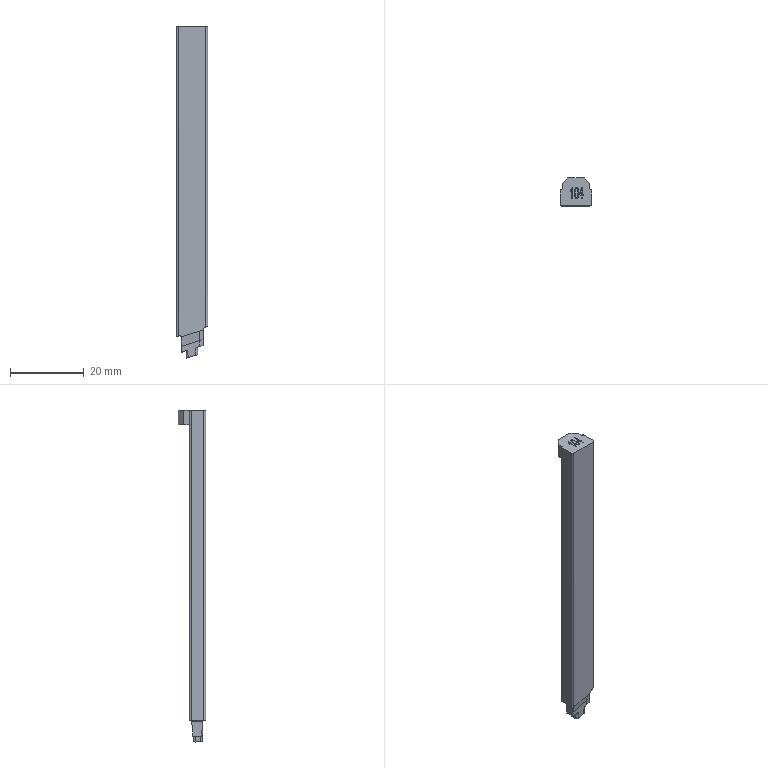Part | Creo | 1 solid | 89 faces | box 8.5 x 7.5 x 90.23 mm | volume 3335 mm3 | plane 43 | other 17 | cylinder 15 | spline 13 | cone 1 | commonest cylinder face diameters 1 x5 1.005 x1 114.945 x1 114.95 x1 116.698 x1 118.069 x1